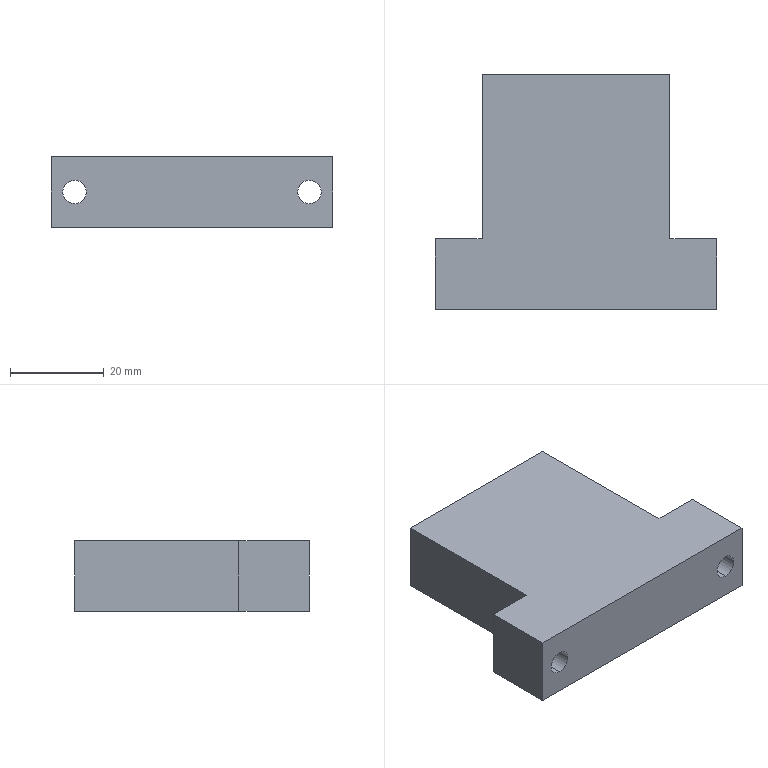Part | STEP file | track spacer block 1 | 1 solid | 26 faces | box 60 x 50 x 15 mm | volume 33797 mm3 | cylinder 10 | plane 10 | cone 6 | commonest cylinder face diameters 2.5 x6 5 x4